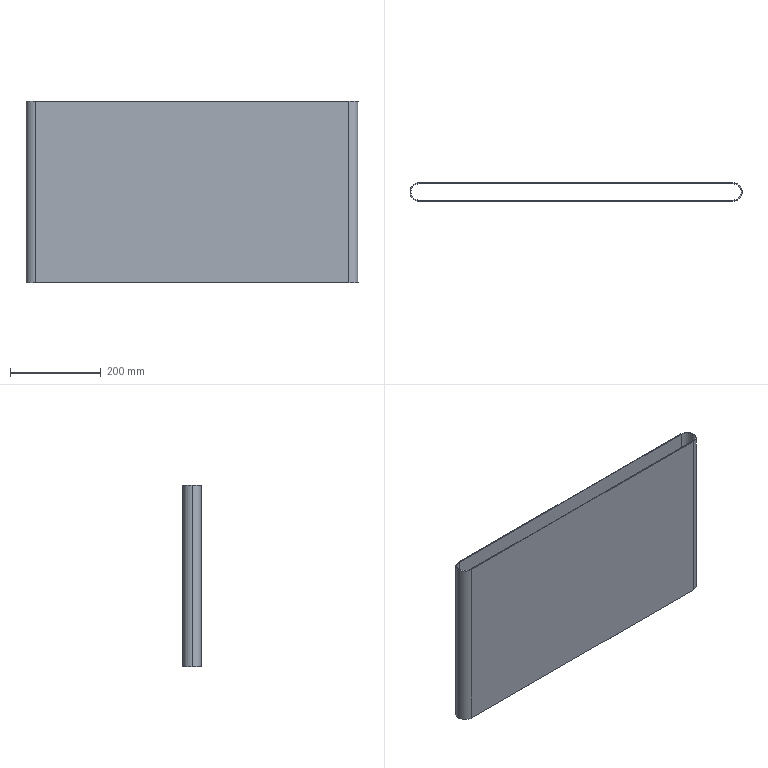Part | STEP file | PN_0019 | 1 solid | 118 faces | box 730 x 40 x 400 mm | volume 1199499 mm3 | plane 69 | spline 43 | cylinder 6 | commonest cylinder face diameters 36 x3 40 x3